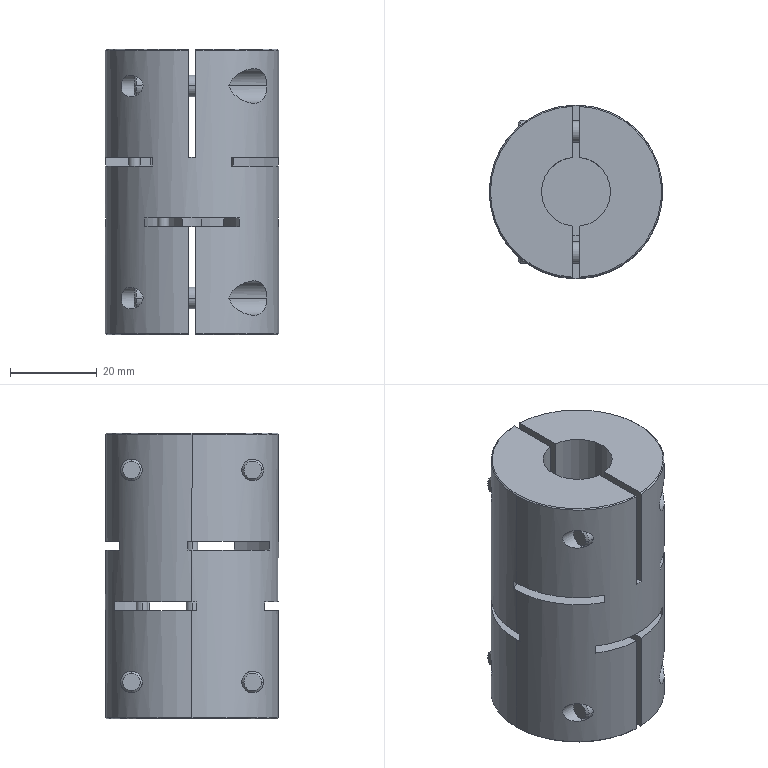Part | STEP file | DCL01-D40-B-d16-e16 | 1 solid | 145 faces | box 40 x 40 x 66 mm | volume 65701 mm3 | cylinder 72 | plane 60 | cone 13 | commonest cylinder face diameters 5 x20 2.667 x12 44 x12 6.667 x8 8 x8 20 x6